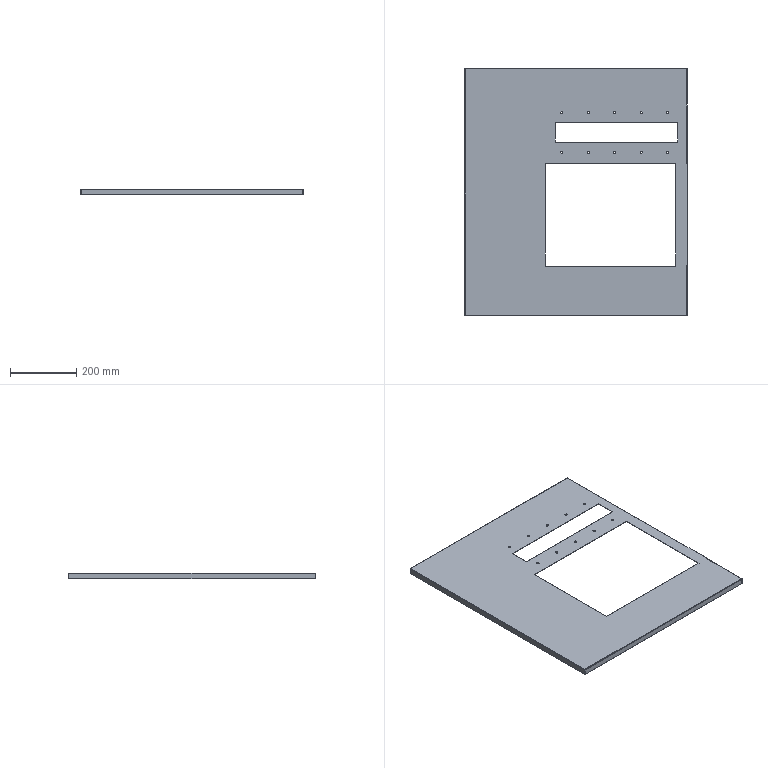Part | SolidWorks | features BaseBody 1 | 1 solid | 83 faces | box 674.5 x 750 x 18 mm | volume 482547 mm3 | plane 47 | cylinder 30 | spline 6 | commonest cylinder face diameters 6.5 x20 1 x5 3.4 x5